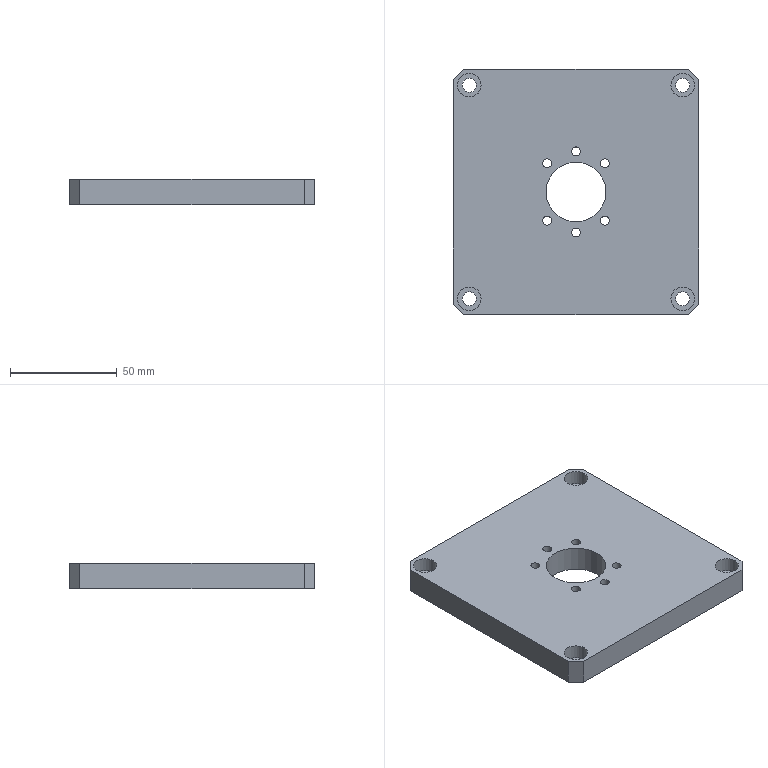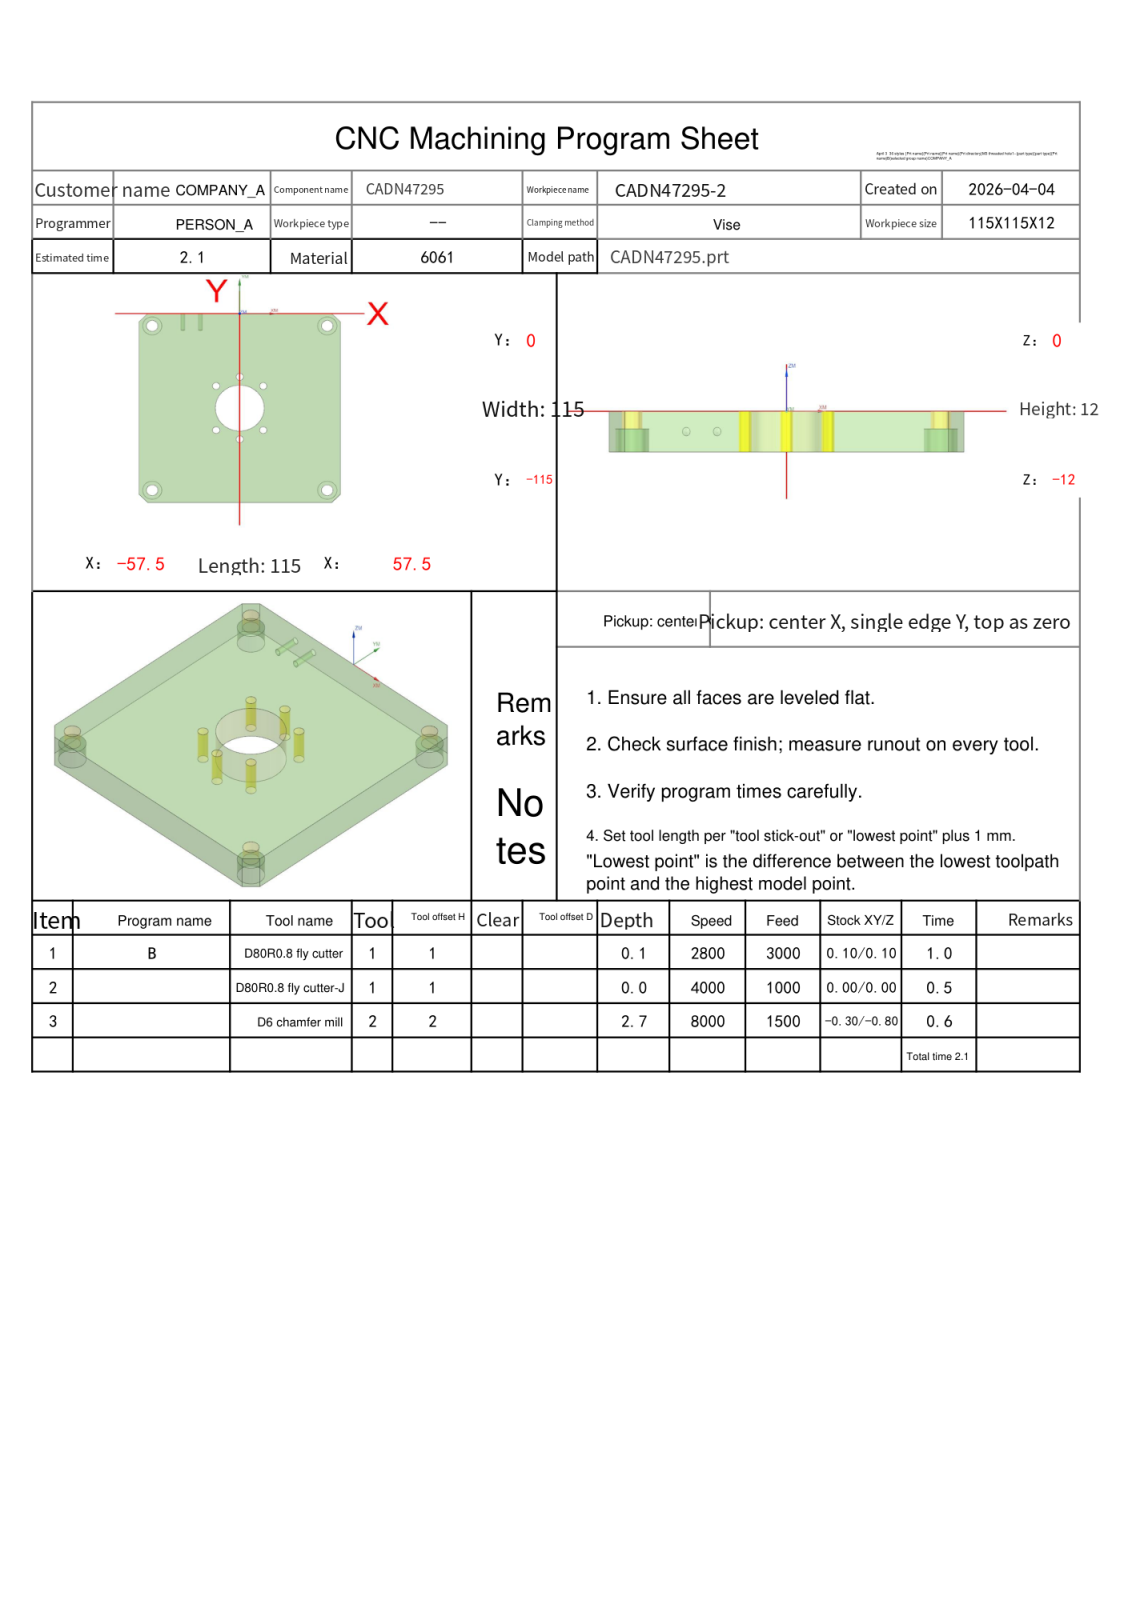NC program | NX | posted by the shop | part box 115 x 115 x 12 mm
Whole program:
%
O0001
(Machine time: 2.60 MIN)
(===Total Tool:2===)
(T1=D80R0.8 fly cutter D=80.  R=0.8  D-  H01 Z=-0.   )
(T2=D6 chamfer mill   D=6.   R=0.   D-  H02 Z=-2.7  )
G80 G90 G17 G49 G40
G91 G28 Z0
M01
N1 T01 M06
(D80R0.8 fly cutter  D=80. R=0.8 H=01 ce=0.10 di=0.10)
G00 G90 G54 X-109.597 Y-23.903 M03 S2800
G43 H01 Z20.
M08
Z4.517
G01 Z2.517 F3000.
X-97.597
X89.6
G02 X97.597 Y-31.901 I-.003 J-8.
G01 Y-75.739
G02 X89.6 Y-83.737 I-8. J.003
G01 X-97.597
X-109.597
Z4.517
G00 Y-23.903
Z4.033
G01 Z2.033
X-97.597
X89.6
G02 X97.597 Y-31.901 I-.003 J-8.
G01 Y-75.739
G02 X89.6 Y-83.737 I-8. J.003
G01 X-97.597
X-109.597
Z4.033
G00 Y-23.903
Z3.55
G01 Z1.55
X-97.597
X89.6
G02 X97.597 Y-31.901 I-.003 J-8.
G01 Y-75.739
G02 X89.6 Y-83.737 I-8. J.003
G01 X-97.597
X-109.597
Z3.55
G00 Y-23.903
Z3.067
G01 Z1.067
X-97.597
X89.6
G02 X97.597 Y-31.901 I-.003 J-8.
G01 Y-75.739
G02 X89.6 Y-83.737 I-8. J.003
G01 X-97.597
X-109.597
Z3.067
G00 Y-23.903
Z2.583
G01 Z.583
X-97.597
X89.6
G02 X97.597 Y-31.901 I-.003 J-8.
G01 Y-75.739
G02 X89.6 Y-83.737 I-8. J.003
G01 X-97.597
X-109.597
Z2.583
G00 Y-23.903
Z2.1
G01 Z.1
X-97.597
X89.6
G02 X97.597 Y-31.901 I-.003 J-8.
G01 Y-75.739
G02 X89.6 Y-83.737 I-8. J.003
G01 X-97.597
X-109.597
Z2.1
G00 Z20.
G91 G28 Z0.0
M05
M09
G91 G28 Z0.0
M01
N2 T01 M06
(D80R0.8 fly cutter-J  D=80. R=0.8 H=01 ce=0.00 di=0.00)
G00 G90 G54 X-109.499 Y-24.001 M03 S4000
G43 H01 Z20.
M08
Z2.
G01 Z0.0 F1000.
X-97.499
X89.502
G02 X97.499 Y-31.998 I-.003 J-8.
G01 Y-75.642
G02 X89.502 Y-83.639 I-8. J.003
G01 X-97.499
X-109.499
Z2.
G00 Z20.
G91 G28 Z0.0
M05
M09
G91 G28 Z0.0
M01
N3 T02 M06
(D6 chamfer mill  D=6. R=0. H=02 ce=0.00 di=0.00)
G00 G90 G54 X-13.435 Y-44.065 M03 S8000
G43 H02 Z20.
M08
G98 G81 X-13.435 Y-44.065 Z-2.7 R3. F1000.
X0.0 Y-38.5
X13.435 Y-44.065
Y-70.935
X0.0 Y-76.5
X-13.435 Y-70.935
G80
G00 Z20.
G00 G90 X50.507 Y-108.587 M03 S8000
Z20.
Z-.9
G01 Z-1.4 F1200.
X50.7 Y-109.
G03 X52.2 Y-107.5 I0.0 J1.5
X50. Y-105.3 I-2.2 J0.0
X47.8 Y-107.5 I0.0 J-2.2
X50. Y-109.7 I2.2 J0.0
X52.2 Y-107.5 I0.0 J2.2
X50.7 Y-106. I-1.5 J0.0
G01 X50.507 Y-106.413
Z-.9
G00 Z20.
Y-8.587
Z-.9
G01 Z-1.4
X50.7 Y-9.
G03 X52.2 Y-7.5 I0.0 J1.5
X50. Y-5.3 I-2.2 J0.0
X47.8 Y-7.5 I0.0 J-2.2
X50. Y-9.7 I2.2 J0.0
X52.2 Y-7.5 I0.0 J2.2
X50.7 Y-6. I-1.5 J0.0
G01 X50.507 Y-6.413
Z-.9
G00 Z20.
X-49.493 Y-8.587
Z-.9
G01 Z-1.4
X-49.3 Y-9.
G03 X-47.8 Y-7.5 I0.0 J1.5
X-50. Y-5.3 I-2.2 J0.0
X-52.2 Y-7.5 I0.0 J-2.2
X-50. Y-9.7 I2.2 J0.0
X-47.8 Y-7.5 I0.0 J2.2
X-49.3 Y-6. I-1.5 J0.0
G01 X-49.493 Y-6.413
Z-.9
G00 Z20.
Y-108.587
Z-.9
G01 Z-1.4
X-49.3 Y-109.
G03 X-47.8 Y-107.5 I0.0 J1.5
X-50. Y-105.3 I-2.2 J0.0
X-52.2 Y-107.5 I0.0 J-2.2
X-50. Y-109.7 I2.2 J0.0
X-47.8 Y-107.5 I0.0 J2.2
X-49.3 Y-106. I-1.5 J0.0
G01 X-49.493 Y-106.413
Z-.9
G00 Z20.
G00 G90 X58.2 Y-101.046 M03 S7000
Z20.
Z2.5
G01 Y-109.953 Z-.742 F1500.
X58.162 Y-110.16 Z-.819
X58.081 Y-110.355 Z-.895
X57.962 Y-110.528 Z-.972
X57.907 Y-110.583 Z-1.
X53.083 Y-115.407
G02 X52.376 Y-115.7 I-.707 J.707
G01 X-52.376
G02 X-53.083 Y-115.407 I0.0 J1.
G01 X-57.907 Y-110.583
G02 X-58.2 Y-109.876 I.707 J.707
G01 Y-5.124
G02 X-57.907 Y-4.417 I1. J0.0
G01 X-53.083 Y.407
G02 X-52.376 Y.7 I.707 J-.707
G01 X52.376
G02 X53.083 Y.407 I0.0 J-1.
G01 X57.907 Y-4.417
G02 X58.2 Y-5.124 I-.707 J-.707
G01 Y-109.876
G02 X57.907 Y-110.583 I-1. J0.0
G01 X57.554 Y-110.936
Z1.5
G00 Z20.
X9.975 Y-66.301
Z2.5
G01 X10.459 Y-65.721 Z2.225
X10.923 Y-65.094 Z1.941
X11.349 Y-64.441 Z1.657
X11.736 Y-63.764 Z1.373
X12.083 Y-63.065 Z1.09
X12.388 Y-62.348 Z.806
X12.651 Y-61.614 Z.522
X12.87 Y-60.865 Z.238
X13.045 Y-60.105 Z-.046
X13.176 Y-59.336 Z-.33
X13.261 Y-58.561 Z-.613
X13.3 Y-57.783 Z-.897
Y-57.5 Z-1.
G03 X0.0 Y-44.2 I-13.3 J0.0
X-13.3 Y-57.5 I0.0 J-13.3
X0.0 Y-70.8 I13.3 J0.0
X13.3 Y-57.5 I0.0 J13.3
X13.291 Y-57. I-13.3 J0.0
G01 Z1.5
G00 Z20.
M05
M09
G91 G28 Z0.0
G91 G28 Y0.0
M30
%